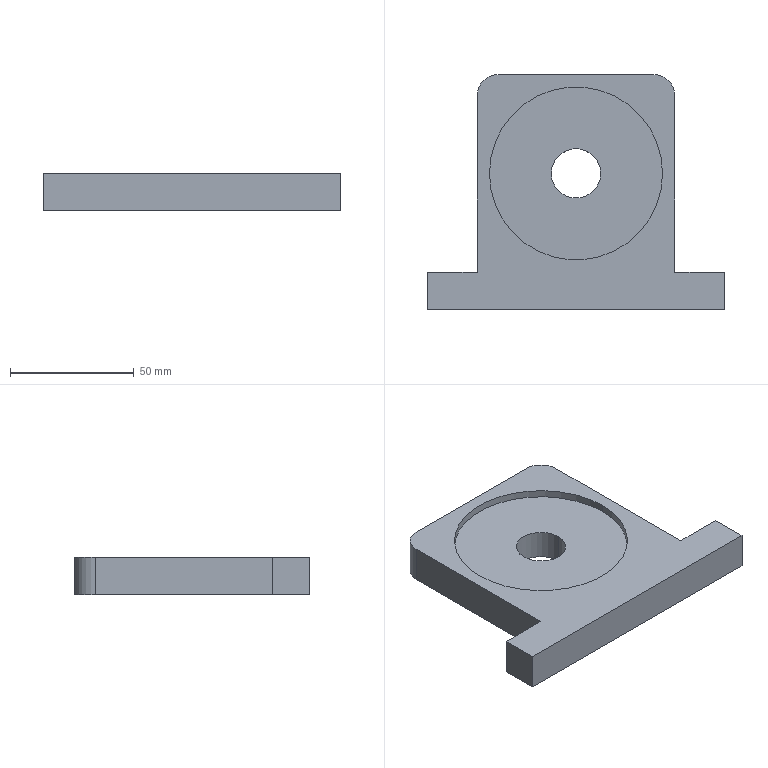Part | SolidWorks | 1 solid | 17 faces | box 120 x 95 x 15 mm | volume 107220 mm3 | plane 11 | cylinder 6 | commonest cylinder face diameters 17 x2 20 x2 70 x2
STEP:
#1=CARTESIAN_POINT('',(-10.,47.5,0.));
#2=VERTEX_POINT('',#1);
#3=CARTESIAN_POINT('',(10.,47.5,0.));
#4=VERTEX_POINT('',#3);
#5=CARTESIAN_POINT('',(0.,47.5,0.));
#6=DIRECTION('',(0.,0.,1.));
#7=DIRECTION('',(1.,0.,0.));
#8=AXIS2_PLACEMENT_3D('',#5,#6,#7);
#9=CIRCLE('',#8,10.);
#10=EDGE_CURVE('',#2,#4,#9,.T.);
#11=ORIENTED_EDGE('',*,*,#10,.F.);
#12=CARTESIAN_POINT('',(-10.,47.5,12.));
#13=VERTEX_POINT('',#12);
#14=CARTESIAN_POINT('',(-10.,47.5,-69.));
#15=DIRECTION('',(0.,0.,1.));
#16=VECTOR('',#15,1000.);
#17=LINE('',#14,#16);
#18=EDGE_CURVE('',#2,#13,#17,.T.);
#19=ORIENTED_EDGE('',*,*,#18,.T.);
#20=CARTESIAN_POINT('',(10.,47.5,12.));
#21=VERTEX_POINT('',#20);
#22=CARTESIAN_POINT('',(0.,47.5,12.));
#23=DIRECTION('',(0.,0.,1.));
#24=DIRECTION('',(1.,0.,0.));
#25=AXIS2_PLACEMENT_3D('',#22,#23,#24);
#26=CIRCLE('',#25,10.);
#27=EDGE_CURVE('',#13,#21,#26,.T.);
#28=ORIENTED_EDGE('',*,*,#27,.T.);
#29=CARTESIAN_POINT('',(10.,47.5,-69.));
#30=DIRECTION('',(0.,0.,1.));
#31=VECTOR('',#30,1000.);
#32=LINE('',#29,#31);
#33=EDGE_CURVE('',#4,#21,#32,.T.);
#34=ORIENTED_EDGE('',*,*,#33,.F.);
#35=EDGE_LOOP('',(#11,#19,#28,#34));
#36=FACE_OUTER_BOUND('',#35,.T.);
#37=CARTESIAN_POINT('',(0.,47.5,-69.));
#38=DIRECTION('',(0.,0.,1.));
#39=DIRECTION('',(1.,0.,0.));
#40=AXIS2_PLACEMENT_3D('',#37,#38,#39);
#41=CYLINDRICAL_SURFACE('',#40,10.);
#42=ADVANCED_FACE('',(#36),#41,.F.);
#43=CARTESIAN_POINT('',(-35.,47.5,12.));
#44=VERTEX_POINT('',#43);
#45=CARTESIAN_POINT('',(35.,47.5,12.));
#46=VERTEX_POINT('',#45);
#47=CARTESIAN_POINT('',(0.,47.5,12.));
#48=DIRECTION('',(0.,0.,1.));
#49=DIRECTION('',(1.,0.,0.));
#50=AXIS2_PLACEMENT_3D('',#47,#48,#49);
#51=CIRCLE('',#50,35.);
#52=EDGE_CURVE('',#44,#46,#51,.T.);
#53=ORIENTED_EDGE('',*,*,#52,.F.);
#54=CARTESIAN_POINT('',(-35.,47.5,15.));
#55=VERTEX_POINT('',#54);
#56=CARTESIAN_POINT('',(-35.,47.5,12.));
#57=DIRECTION('',(0.,0.,1.));
#58=VECTOR('',#57,1000.);
#59=LINE('',#56,#58);
#60=EDGE_CURVE('',#44,#55,#59,.T.);
#61=ORIENTED_EDGE('',*,*,#60,.T.);
#62=CARTESIAN_POINT('',(35.,47.5,15.));
#63=VERTEX_POINT('',#62);
#64=CARTESIAN_POINT('',(0.,47.5,15.));
#65=DIRECTION('',(0.,0.,1.));
#66=DIRECTION('',(1.,0.,0.));
#67=AXIS2_PLACEMENT_3D('',#64,#65,#66);
#68=CIRCLE('',#67,35.);
#69=EDGE_CURVE('',#55,#63,#68,.T.);
#70=ORIENTED_EDGE('',*,*,#69,.T.);
#71=CARTESIAN_POINT('',(35.,47.5,12.));
#72=DIRECTION('',(0.,0.,1.));
#73=VECTOR('',#72,1000.);
#74=LINE('',#71,#73);
#75=EDGE_CURVE('',#46,#63,#74,.T.);
#76=ORIENTED_EDGE('',*,*,#75,.F.);
#77=EDGE_LOOP('',(#53,#61,#70,#76));
#78=FACE_OUTER_BOUND('',#77,.T.);
#79=CARTESIAN_POINT('',(0.,47.5,12.));
#80=DIRECTION('',(0.,0.,1.));
#81=DIRECTION('',(1.,0.,0.));
#82=AXIS2_PLACEMENT_3D('',#79,#80,#81);
#83=CYLINDRICAL_SURFACE('',#82,35.);
#84=ADVANCED_FACE('',(#78),#83,.F.);
#85=CARTESIAN_POINT('',(60.,-7.5,0.));
#86=VERTEX_POINT('',#85);
#87=CARTESIAN_POINT('',(60.,7.5,0.));
#88=VERTEX_POINT('',#87);
#89=CARTESIAN_POINT('',(60.,7.5,0.));
#90=DIRECTION('',(0.,1.,0.));
#91=VECTOR('',#90,1000.);
#92=LINE('',#89,#91);
#93=EDGE_CURVE('',#86,#88,#92,.T.);
#94=ORIENTED_EDGE('',*,*,#93,.T.);
#95=CARTESIAN_POINT('',(60.,7.5,15.));
#96=VERTEX_POINT('',#95);
#97=CARTESIAN_POINT('',(60.,7.5,15.));
#98=DIRECTION('',(0.,0.,-1.));
#99=VECTOR('',#98,1000.);
#100=LINE('',#97,#99);
#101=EDGE_CURVE('',#96,#88,#100,.T.);
#102=ORIENTED_EDGE('',*,*,#101,.F.);
#103=CARTESIAN_POINT('',(60.,-7.5,15.));
#104=VERTEX_POINT('',#103);
#105=CARTESIAN_POINT('',(60.,7.5,15.));
#106=DIRECTION('',(0.,1.,0.));
#107=VECTOR('',#106,1000.);
#108=LINE('',#105,#107);
#109=EDGE_CURVE('',#104,#96,#108,.T.);
#110=ORIENTED_EDGE('',*,*,#109,.F.);
#111=CARTESIAN_POINT('',(60.,-7.5,15.));
#112=DIRECTION('',(0.,0.,-1.));
#113=VECTOR('',#112,1000.);
#114=LINE('',#111,#113);
#115=EDGE_CURVE('',#104,#86,#114,.T.);
#116=ORIENTED_EDGE('',*,*,#115,.T.);
#117=EDGE_LOOP('',(#94,#102,#110,#116));
#118=FACE_OUTER_BOUND('',#117,.T.);
#119=CARTESIAN_POINT('',(60.,7.5,15.));
#120=DIRECTION('',(-1.,0.,0.));
#121=DIRECTION('',(0.,-1.,0.));
#122=AXIS2_PLACEMENT_3D('',#119,#120,#121);
#123=PLANE('',#122);
#124=ADVANCED_FACE('',(#118),#123,.F.);
#125=CARTESIAN_POINT('',(40.,7.5,0.));
#126=VERTEX_POINT('',#125);
#127=CARTESIAN_POINT('',(40.,7.5,0.));
#128=DIRECTION('',(-1.,0.,0.));
#129=VECTOR('',#128,1000.);
#130=LINE('',#127,#129);
#131=EDGE_CURVE('',#88,#126,#130,.T.);
#132=ORIENTED_EDGE('',*,*,#131,.T.);
#133=CARTESIAN_POINT('',(40.,7.5,15.));
#134=VERTEX_POINT('',#133);
#135=CARTESIAN_POINT('',(40.,7.5,15.));
#136=DIRECTION('',(0.,0.,-1.));
#137=VECTOR('',#136,1000.);
#138=LINE('',#135,#137);
#139=EDGE_CURVE('',#134,#126,#138,.T.);
#140=ORIENTED_EDGE('',*,*,#139,.F.);
#141=CARTESIAN_POINT('',(40.,7.5,15.));
#142=DIRECTION('',(-1.,0.,0.));
#143=VECTOR('',#142,1000.);
#144=LINE('',#141,#143);
#145=EDGE_CURVE('',#96,#134,#144,.T.);
#146=ORIENTED_EDGE('',*,*,#145,.F.);
#147=ORIENTED_EDGE('',*,*,#101,.T.);
#148=EDGE_LOOP('',(#132,#140,#146,#147));
#149=FACE_OUTER_BOUND('',#148,.T.);
#150=CARTESIAN_POINT('',(40.,7.5,15.));
#151=DIRECTION('',(0.,-1.,0.));
#152=DIRECTION('',(1.,0.,0.));
#153=AXIS2_PLACEMENT_3D('',#150,#151,#152);
#154=PLANE('',#153);
#155=ADVANCED_FACE('',(#149),#154,.F.);
#156=CARTESIAN_POINT('',(40.,79.,0.));
#157=VERTEX_POINT('',#156);
#158=CARTESIAN_POINT('',(40.,7.5,0.));
#159=DIRECTION('',(0.,1.,0.));
#160=VECTOR('',#159,1000.);
#161=LINE('',#158,#160);
#162=EDGE_CURVE('',#126,#157,#161,.T.);
#163=ORIENTED_EDGE('',*,*,#162,.T.);
#164=CARTESIAN_POINT('',(40.,79.,15.));
#165=VERTEX_POINT('',#164);
#166=CARTESIAN_POINT('',(40.,79.,15.));
#167=DIRECTION('',(0.,0.,1.));
#168=VECTOR('',#167,1000.);
#169=LINE('',#166,#168);
#170=EDGE_CURVE('',#157,#165,#169,.T.);
#171=ORIENTED_EDGE('',*,*,#170,.T.);
#172=CARTESIAN_POINT('',(40.,7.5,15.));
#173=DIRECTION('',(0.,1.,0.));
#174=VECTOR('',#173,1000.);
#175=LINE('',#172,#174);
#176=EDGE_CURVE('',#134,#165,#175,.T.);
#177=ORIENTED_EDGE('',*,*,#176,.F.);
#178=ORIENTED_EDGE('',*,*,#139,.T.);
#179=EDGE_LOOP('',(#163,#171,#177,#178));
#180=FACE_OUTER_BOUND('',#179,.T.);
#181=CARTESIAN_POINT('',(40.,7.5,15.));
#182=DIRECTION('',(-1.,0.,0.));
#183=DIRECTION('',(0.,-1.,0.));
#184=AXIS2_PLACEMENT_3D('',#181,#182,#183);
#185=PLANE('',#184);
#186=ADVANCED_FACE('',(#180),#185,.F.);
#187=CARTESIAN_POINT('',(31.5,87.5,15.));
#188=VERTEX_POINT('',#187);
#189=CARTESIAN_POINT('',(-31.5,87.5,15.));
#190=VERTEX_POINT('',#189);
#191=CARTESIAN_POINT('',(-40.,87.5,15.));
#192=DIRECTION('',(-1.,0.,0.));
#193=VECTOR('',#192,1000.);
#194=LINE('',#191,#193);
#195=EDGE_CURVE('',#188,#190,#194,.T.);
#196=ORIENTED_EDGE('',*,*,#195,.F.);
#197=CARTESIAN_POINT('',(31.5,87.5,0.));
#198=VERTEX_POINT('',#197);
#199=CARTESIAN_POINT('',(31.5,87.5,15.));
#200=DIRECTION('',(0.,0.,-1.));
#201=VECTOR('',#200,1000.);
#202=LINE('',#199,#201);
#203=EDGE_CURVE('',#188,#198,#202,.T.);
#204=ORIENTED_EDGE('',*,*,#203,.T.);
#205=CARTESIAN_POINT('',(-31.5,87.5,0.));
#206=VERTEX_POINT('',#205);
#207=CARTESIAN_POINT('',(-40.,87.5,0.));
#208=DIRECTION('',(-1.,0.,0.));
#209=VECTOR('',#208,1000.);
#210=LINE('',#207,#209);
#211=EDGE_CURVE('',#198,#206,#210,.T.);
#212=ORIENTED_EDGE('',*,*,#211,.T.);
#213=CARTESIAN_POINT('',(-31.5,87.5,15.));
#214=DIRECTION('',(0.,0.,1.));
#215=VECTOR('',#214,1000.);
#216=LINE('',#213,#215);
#217=EDGE_CURVE('',#206,#190,#216,.T.);
#218=ORIENTED_EDGE('',*,*,#217,.T.);
#219=EDGE_LOOP('',(#196,#204,#212,#218));
#220=FACE_OUTER_BOUND('',#219,.T.);
#221=CARTESIAN_POINT('',(-40.,87.5,15.));
#222=DIRECTION('',(0.,-1.,0.));
#223=DIRECTION('',(0.,0.,-1.));
#224=AXIS2_PLACEMENT_3D('',#221,#222,#223);
#225=PLANE('',#224);
#226=ADVANCED_FACE('',(#220),#225,.F.);
#227=CARTESIAN_POINT('',(-40.,79.,15.));
#228=VERTEX_POINT('',#227);
#229=CARTESIAN_POINT('',(-40.,7.5,15.));
#230=VERTEX_POINT('',#229);
#231=CARTESIAN_POINT('',(-40.,7.5,15.));
#232=DIRECTION('',(0.,-1.,0.));
#233=VECTOR('',#232,1000.);
#234=LINE('',#231,#233);
#235=EDGE_CURVE('',#228,#230,#234,.T.);
#236=ORIENTED_EDGE('',*,*,#235,.F.);
#237=CARTESIAN_POINT('',(-40.,79.,0.));
#238=VERTEX_POINT('',#237);
#239=CARTESIAN_POINT('',(-40.,79.,15.));
#240=DIRECTION('',(0.,0.,-1.));
#241=VECTOR('',#240,1000.);
#242=LINE('',#239,#241);
#243=EDGE_CURVE('',#228,#238,#242,.T.);
#244=ORIENTED_EDGE('',*,*,#243,.T.);
#245=CARTESIAN_POINT('',(-40.,7.5,0.));
#246=VERTEX_POINT('',#245);
#247=CARTESIAN_POINT('',(-40.,7.5,0.));
#248=DIRECTION('',(0.,-1.,0.));
#249=VECTOR('',#248,1000.);
#250=LINE('',#247,#249);
#251=EDGE_CURVE('',#238,#246,#250,.T.);
#252=ORIENTED_EDGE('',*,*,#251,.T.);
#253=CARTESIAN_POINT('',(-40.,7.5,15.));
#254=DIRECTION('',(0.,0.,-1.));
#255=VECTOR('',#254,1000.);
#256=LINE('',#253,#255);
#257=EDGE_CURVE('',#230,#246,#256,.T.);
#258=ORIENTED_EDGE('',*,*,#257,.F.);
#259=EDGE_LOOP('',(#236,#244,#252,#258));
#260=FACE_OUTER_BOUND('',#259,.T.);
#261=CARTESIAN_POINT('',(-40.,7.5,15.));
#262=DIRECTION('',(1.,0.,0.));
#263=DIRECTION('',(0.,1.,0.));
#264=AXIS2_PLACEMENT_3D('',#261,#262,#263);
#265=PLANE('',#264);
#266=ADVANCED_FACE('',(#260),#265,.F.);
#267=CARTESIAN_POINT('',(-60.,7.5,0.));
#268=VERTEX_POINT('',#267);
#269=CARTESIAN_POINT('',(-60.,7.5,0.));
#270=DIRECTION('',(-1.,0.,0.));
#271=VECTOR('',#270,1000.);
#272=LINE('',#269,#271);
#273=EDGE_CURVE('',#246,#268,#272,.T.);
#274=ORIENTED_EDGE('',*,*,#273,.T.);
#275=CARTESIAN_POINT('',(-60.,7.5,15.));
#276=VERTEX_POINT('',#275);
#277=CARTESIAN_POINT('',(-60.,7.5,15.));
#278=DIRECTION('',(0.,0.,-1.));
#279=VECTOR('',#278,1000.);
#280=LINE('',#277,#279);
#281=EDGE_CURVE('',#276,#268,#280,.T.);
#282=ORIENTED_EDGE('',*,*,#281,.F.);
#283=CARTESIAN_POINT('',(-60.,7.5,15.));
#284=DIRECTION('',(-1.,0.,0.));
#285=VECTOR('',#284,1000.);
#286=LINE('',#283,#285);
#287=EDGE_CURVE('',#230,#276,#286,.T.);
#288=ORIENTED_EDGE('',*,*,#287,.F.);
#289=ORIENTED_EDGE('',*,*,#257,.T.);
#290=EDGE_LOOP('',(#274,#282,#288,#289));
#291=FACE_OUTER_BOUND('',#290,.T.);
#292=CARTESIAN_POINT('',(-60.,7.5,15.));
#293=DIRECTION('',(0.,-1.,0.));
#294=DIRECTION('',(1.,0.,0.));
#295=AXIS2_PLACEMENT_3D('',#292,#293,#294);
#296=PLANE('',#295);
#297=ADVANCED_FACE('',(#291),#296,.F.);
#298=CARTESIAN_POINT('',(-60.,-7.5,0.));
#299=VERTEX_POINT('',#298);
#300=CARTESIAN_POINT('',(-60.,7.5,0.));
#301=DIRECTION('',(0.,-1.,0.));
#302=VECTOR('',#301,1000.);
#303=LINE('',#300,#302);
#304=EDGE_CURVE('',#268,#299,#303,.T.);
#305=ORIENTED_EDGE('',*,*,#304,.T.);
#306=CARTESIAN_POINT('',(-60.,-7.5,15.));
#307=VERTEX_POINT('',#306);
#308=CARTESIAN_POINT('',(-60.,-7.5,15.));
#309=DIRECTION('',(0.,0.,-1.));
#310=VECTOR('',#309,1000.);
#311=LINE('',#308,#310);
#312=EDGE_CURVE('',#307,#299,#311,.T.);
#313=ORIENTED_EDGE('',*,*,#312,.F.);
#314=CARTESIAN_POINT('',(-60.,7.5,15.));
#315=DIRECTION('',(0.,-1.,0.));
#316=VECTOR('',#315,1000.);
#317=LINE('',#314,#316);
#318=EDGE_CURVE('',#276,#307,#317,.T.);
#319=ORIENTED_EDGE('',*,*,#318,.F.);
#320=ORIENTED_EDGE('',*,*,#281,.T.);
#321=EDGE_LOOP('',(#305,#313,#319,#320));
#322=FACE_OUTER_BOUND('',#321,.T.);
#323=CARTESIAN_POINT('',(-60.,7.5,15.));
#324=DIRECTION('',(1.,0.,0.));
#325=DIRECTION('',(0.,0.,-1.));
#326=AXIS2_PLACEMENT_3D('',#323,#324,#325);
#327=PLANE('',#326);
#328=ADVANCED_FACE('',(#322),#327,.F.);
#329=CARTESIAN_POINT('',(-60.,-7.5,0.));
#330=DIRECTION('',(1.,0.,0.));
#331=VECTOR('',#330,1000.);
#332=LINE('',#329,#331);
#333=EDGE_CURVE('',#299,#86,#332,.T.);
#334=ORIENTED_EDGE('',*,*,#333,.T.);
#335=ORIENTED_EDGE('',*,*,#115,.F.);
#336=CARTESIAN_POINT('',(-60.,-7.5,15.));
#337=DIRECTION('',(1.,0.,0.));
#338=VECTOR('',#337,1000.);
#339=LINE('',#336,#338);
#340=EDGE_CURVE('',#307,#104,#339,.T.);
#341=ORIENTED_EDGE('',*,*,#340,.F.);
#342=ORIENTED_EDGE('',*,*,#312,.T.);
#343=EDGE_LOOP('',(#334,#335,#341,#342));
#344=FACE_OUTER_BOUND('',#343,.T.);
#345=CARTESIAN_POINT('',(-60.,-7.5,15.));
#346=DIRECTION('',(0.,1.,0.));
#347=DIRECTION('',(-1.,0.,0.));
#348=AXIS2_PLACEMENT_3D('',#345,#346,#347);
#349=PLANE('',#348);
#350=ADVANCED_FACE('',(#344),#349,.F.);
#351=CARTESIAN_POINT('',(0.,47.5,15.));
#352=DIRECTION('',(0.,0.,1.));
#353=DIRECTION('',(1.,0.,0.));
#354=AXIS2_PLACEMENT_3D('',#351,#352,#353);
#355=CIRCLE('',#354,35.);
#356=EDGE_CURVE('',#63,#55,#355,.T.);
#357=ORIENTED_EDGE('',*,*,#356,.F.);
#358=ORIENTED_EDGE('',*,*,#69,.F.);
#359=EDGE_LOOP('',(#357,#358));
#360=FACE_BOUND('',#359,.T.);
#361=ORIENTED_EDGE('',*,*,#176,.T.);
#362=CARTESIAN_POINT('',(31.5,79.,15.));
#363=DIRECTION('',(0.,0.,1.));
#364=DIRECTION('',(1.,0.,0.));
#365=AXIS2_PLACEMENT_3D('',#362,#363,#364);
#366=CIRCLE('',#365,8.5);
#367=EDGE_CURVE('',#165,#188,#366,.T.);
#368=ORIENTED_EDGE('',*,*,#367,.T.);
#369=ORIENTED_EDGE('',*,*,#195,.T.);
#370=CARTESIAN_POINT('',(-31.5,79.,15.));
#371=DIRECTION('',(0.,0.,1.));
#372=DIRECTION('',(1.,0.,0.));
#373=AXIS2_PLACEMENT_3D('',#370,#371,#372);
#374=CIRCLE('',#373,8.5);
#375=EDGE_CURVE('',#190,#228,#374,.T.);
#376=ORIENTED_EDGE('',*,*,#375,.T.);
#377=ORIENTED_EDGE('',*,*,#235,.T.);
#378=ORIENTED_EDGE('',*,*,#287,.T.);
#379=ORIENTED_EDGE('',*,*,#318,.T.);
#380=ORIENTED_EDGE('',*,*,#340,.T.);
#381=ORIENTED_EDGE('',*,*,#109,.T.);
#382=ORIENTED_EDGE('',*,*,#145,.T.);
#383=EDGE_LOOP('',(#361,#368,#369,#376,#377,#378,#379,#380,#381,#382));
#384=FACE_OUTER_BOUND('',#383,.T.);
#385=CARTESIAN_POINT('',(0.,0.,15.));
#386=DIRECTION('',(0.,0.,1.));
#387=DIRECTION('',(1.,0.,0.));
#388=AXIS2_PLACEMENT_3D('',#385,#386,#387);
#389=PLANE('',#388);
#390=ADVANCED_FACE('',(#360,#384),#389,.T.);
#391=CARTESIAN_POINT('',(0.,47.5,0.));
#392=DIRECTION('',(0.,0.,1.));
#393=DIRECTION('',(1.,0.,0.));
#394=AXIS2_PLACEMENT_3D('',#391,#392,#393);
#395=CIRCLE('',#394,10.);
#396=EDGE_CURVE('',#4,#2,#395,.T.);
#397=ORIENTED_EDGE('',*,*,#396,.T.);
#398=ORIENTED_EDGE('',*,*,#10,.T.);
#399=EDGE_LOOP('',(#397,#398));
#400=FACE_BOUND('',#399,.T.);
#401=ORIENTED_EDGE('',*,*,#211,.F.);
#402=CARTESIAN_POINT('',(31.5,79.,0.));
#403=DIRECTION('',(0.,0.,-1.));
#404=DIRECTION('',(1.,0.,0.));
#405=AXIS2_PLACEMENT_3D('',#402,#403,#404);
#406=CIRCLE('',#405,8.5);
#407=EDGE_CURVE('',#198,#157,#406,.T.);
#408=ORIENTED_EDGE('',*,*,#407,.T.);
#409=ORIENTED_EDGE('',*,*,#162,.F.);
#410=ORIENTED_EDGE('',*,*,#131,.F.);
#411=ORIENTED_EDGE('',*,*,#93,.F.);
#412=ORIENTED_EDGE('',*,*,#333,.F.);
#413=ORIENTED_EDGE('',*,*,#304,.F.);
#414=ORIENTED_EDGE('',*,*,#273,.F.);
#415=ORIENTED_EDGE('',*,*,#251,.F.);
#416=CARTESIAN_POINT('',(-31.5,79.,0.));
#417=DIRECTION('',(0.,0.,-1.));
#418=DIRECTION('',(1.,0.,0.));
#419=AXIS2_PLACEMENT_3D('',#416,#417,#418);
#420=CIRCLE('',#419,8.5);
#421=EDGE_CURVE('',#238,#206,#420,.T.);
#422=ORIENTED_EDGE('',*,*,#421,.T.);
#423=EDGE_LOOP('',(#401,#408,#409,#410,#411,#412,#413,#414,#415,#422));
#424=FACE_OUTER_BOUND('',#423,.T.);
#425=CARTESIAN_POINT('',(0.,0.,0.));
#426=DIRECTION('',(0.,0.,1.));
#427=DIRECTION('',(1.,0.,0.));
#428=AXIS2_PLACEMENT_3D('',#425,#426,#427);
#429=PLANE('',#428);
#430=ADVANCED_FACE('',(#400,#424),#429,.F.);
#431=ORIENTED_EDGE('',*,*,#60,.F.);
#432=CARTESIAN_POINT('',(0.,47.5,12.));
#433=DIRECTION('',(0.,0.,1.));
#434=DIRECTION('',(1.,0.,0.));
#435=AXIS2_PLACEMENT_3D('',#432,#433,#434);
#436=CIRCLE('',#435,35.);
#437=EDGE_CURVE('',#46,#44,#436,.T.);
#438=ORIENTED_EDGE('',*,*,#437,.F.);
#439=ORIENTED_EDGE('',*,*,#75,.T.);
#440=ORIENTED_EDGE('',*,*,#356,.T.);
#441=EDGE_LOOP('',(#431,#438,#439,#440));
#442=FACE_OUTER_BOUND('',#441,.T.);
#443=CARTESIAN_POINT('',(0.,47.5,12.));
#444=DIRECTION('',(0.,0.,1.));
#445=DIRECTION('',(1.,0.,0.));
#446=AXIS2_PLACEMENT_3D('',#443,#444,#445);
#447=CYLINDRICAL_SURFACE('',#446,35.);
#448=ADVANCED_FACE('',(#442),#447,.F.);
#449=CARTESIAN_POINT('',(0.,47.5,12.));
#450=DIRECTION('',(0.,0.,1.));
#451=DIRECTION('',(1.,0.,0.));
#452=AXIS2_PLACEMENT_3D('',#449,#450,#451);
#453=CIRCLE('',#452,10.);
#454=EDGE_CURVE('',#21,#13,#453,.T.);
#455=ORIENTED_EDGE('',*,*,#454,.F.);
#456=ORIENTED_EDGE('',*,*,#27,.F.);
#457=EDGE_LOOP('',(#455,#456));
#458=FACE_BOUND('',#457,.T.);
#459=ORIENTED_EDGE('',*,*,#437,.T.);
#460=ORIENTED_EDGE('',*,*,#52,.T.);
#461=EDGE_LOOP('',(#459,#460));
#462=FACE_OUTER_BOUND('',#461,.T.);
#463=CARTESIAN_POINT('',(0.,47.5,12.));
#464=DIRECTION('',(0.,0.,1.));
#465=DIRECTION('',(1.,0.,0.));
#466=AXIS2_PLACEMENT_3D('',#463,#464,#465);
#467=PLANE('',#466);
#468=ADVANCED_FACE('',(#458,#462),#467,.T.);
#469=ORIENTED_EDGE('',*,*,#18,.F.);
#470=ORIENTED_EDGE('',*,*,#396,.F.);
#471=ORIENTED_EDGE('',*,*,#33,.T.);
#472=ORIENTED_EDGE('',*,*,#454,.T.);
#473=EDGE_LOOP('',(#469,#470,#471,#472));
#474=FACE_OUTER_BOUND('',#473,.T.);
#475=CARTESIAN_POINT('',(0.,47.5,-69.));
#476=DIRECTION('',(0.,0.,1.));
#477=DIRECTION('',(1.,0.,0.));
#478=AXIS2_PLACEMENT_3D('',#475,#476,#477);
#479=CYLINDRICAL_SURFACE('',#478,10.);
#480=ADVANCED_FACE('',(#474),#479,.F.);
#481=ORIENTED_EDGE('',*,*,#367,.F.);
#482=ORIENTED_EDGE('',*,*,#170,.F.);
#483=ORIENTED_EDGE('',*,*,#407,.F.);
#484=ORIENTED_EDGE('',*,*,#203,.F.);
#485=EDGE_LOOP('',(#481,#482,#483,#484));
#486=FACE_OUTER_BOUND('',#485,.T.);
#487=CARTESIAN_POINT('',(31.5,79.,15.));
#488=DIRECTION('',(0.,0.,-1.));
#489=DIRECTION('',(-1.,0.,0.));
#490=AXIS2_PLACEMENT_3D('',#487,#488,#489);
#491=CYLINDRICAL_SURFACE('',#490,8.5);
#492=ADVANCED_FACE('',(#486),#491,.T.);
#493=ORIENTED_EDGE('',*,*,#375,.F.);
#494=ORIENTED_EDGE('',*,*,#217,.F.);
#495=ORIENTED_EDGE('',*,*,#421,.F.);
#496=ORIENTED_EDGE('',*,*,#243,.F.);
#497=EDGE_LOOP('',(#493,#494,#495,#496));
#498=FACE_OUTER_BOUND('',#497,.T.);
#499=CARTESIAN_POINT('',(-31.5,79.,15.));
#500=DIRECTION('',(0.,0.,-1.));
#501=DIRECTION('',(-1.,0.,0.));
#502=AXIS2_PLACEMENT_3D('',#499,#500,#501);
#503=CYLINDRICAL_SURFACE('',#502,8.5);
#504=ADVANCED_FACE('',(#498),#503,.T.);
#505=CLOSED_SHELL('',(#42,#84,#124,#155,#186,#226,#266,#297,#328,#350,#390,#430,#448,#468,#480,#492,#504));
#506=MANIFOLD_SOLID_BREP('',#505);
#507=CARTESIAN_POINT('',(0.,0.,0.));
#508=DIRECTION('',(0.,0.,1.));
#509=DIRECTION('',(1.,0.,0.));
#510=AXIS2_PLACEMENT_3D('',#507,#508,#509);
#511=(LENGTH_UNIT()NAMED_UNIT(*)SI_UNIT(.MILLI.,.METRE.));
#512=UNCERTAINTY_MEASURE_WITH_UNIT(LENGTH_MEASURE(0.00001),#511,'','');
#513=(NAMED_UNIT(*)PLANE_ANGLE_UNIT()SI_UNIT($,.RADIAN.));
#514=(NAMED_UNIT(*)SI_UNIT($,.STERADIAN.)SOLID_ANGLE_UNIT());
#515=(GEOMETRIC_REPRESENTATION_CONTEXT(3)GLOBAL_UNCERTAINTY_ASSIGNED_CONTEXT((#512))GLOBAL_UNIT_ASSIGNED_CONTEXT((#511,#513,#514))REPRESENTATION_CONTEXT('',''));
#516=ADVANCED_BREP_SHAPE_REPRESENTATION('',(#506,#510),#515);